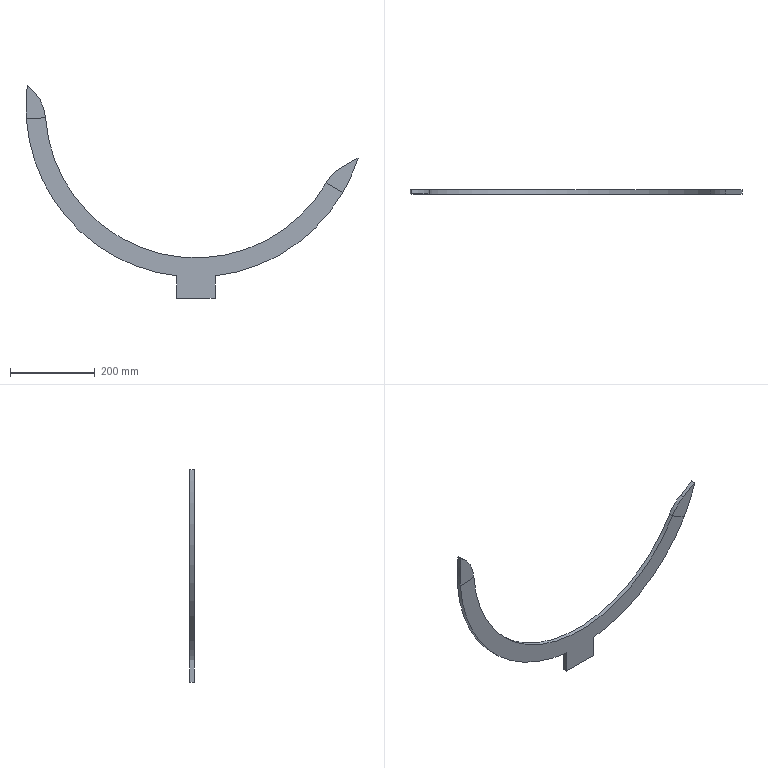Part | NX | features DATUM_CSYS 2, DIVIDE_FACE 1, EXTRUDE 1, SKETCH 1 | 1 solid | 15 faces | box 781.576 x 10 x 500 mm | volume 527562 mm3 | plane 10 | cylinder 5 | commonest cylinder face diameters 200 x2 800 x2 710 x1
STEP:
#1=CARTESIAN_POINT('',(-354.112,-5.,-25.096));
#2=VERTEX_POINT('',#1);
#3=CARTESIAN_POINT('',(306.914,-5.,-178.406));
#4=VERTEX_POINT('',#3);
#5=CARTESIAN_POINT('',(0.,-5.,0.));
#6=DIRECTION('',(0.,1.,0.));
#7=DIRECTION('',(1.,0.,0.));
#8=AXIS2_PLACEMENT_3D('',#5,#6,#7);
#9=CIRCLE('',#8,355.);
#10=EDGE_CURVE('',#2,#4,#9,.F.);
#11=ORIENTED_EDGE('',*,*,#10,.F.);
#12=CARTESIAN_POINT('',(-398.999,-5.,-28.277));
#13=VERTEX_POINT('',#12);
#14=CARTESIAN_POINT('',(-354.112,-5.,-25.096));
#15=DIRECTION('',(-0.9975,0.,-0.07069));
#16=VECTOR('',#15,1000.);
#17=LINE('',#14,#16);
#18=EDGE_CURVE('',#2,#13,#17,.T.);
#19=ORIENTED_EDGE('',*,*,#18,.T.);
#20=CARTESIAN_POINT('',(-45.,-5.,-397.461));
#21=VERTEX_POINT('',#20);
#22=CARTESIAN_POINT('',(0.,-5.,0.));
#23=DIRECTION('',(0.,-1.,0.));
#24=DIRECTION('',(1.,0.,0.));
#25=AXIS2_PLACEMENT_3D('',#22,#23,#24);
#26=CIRCLE('',#25,400.);
#27=EDGE_CURVE('',#21,#13,#26,.F.);
#28=ORIENTED_EDGE('',*,*,#27,.F.);
#29=CARTESIAN_POINT('',(-45.,-5.,-450.));
#30=VERTEX_POINT('',#29);
#31=CARTESIAN_POINT('',(-45.,-5.,-397.461));
#32=DIRECTION('',(0.,0.,-1.));
#33=VECTOR('',#32,1000.);
#34=LINE('',#31,#33);
#35=EDGE_CURVE('',#30,#21,#34,.F.);
#36=ORIENTED_EDGE('',*,*,#35,.F.);
#37=CARTESIAN_POINT('',(45.,-5.,-450.));
#38=VERTEX_POINT('',#37);
#39=CARTESIAN_POINT('',(-45.,-5.,-450.));
#40=DIRECTION('',(1.,0.,0.));
#41=VECTOR('',#40,1000.);
#42=LINE('',#39,#41);
#43=EDGE_CURVE('',#38,#30,#42,.F.);
#44=ORIENTED_EDGE('',*,*,#43,.F.);
#45=CARTESIAN_POINT('',(45.,-5.,-397.461));
#46=VERTEX_POINT('',#45);
#47=CARTESIAN_POINT('',(45.,-5.,-450.));
#48=DIRECTION('',(0.,0.,1.));
#49=VECTOR('',#48,1000.);
#50=LINE('',#47,#49);
#51=EDGE_CURVE('',#46,#38,#50,.F.);
#52=ORIENTED_EDGE('',*,*,#51,.F.);
#53=CARTESIAN_POINT('',(345.819,-5.,-201.021));
#54=VERTEX_POINT('',#53);
#55=CARTESIAN_POINT('',(0.,-5.,0.));
#56=DIRECTION('',(0.,-1.,0.));
#57=DIRECTION('',(1.,0.,0.));
#58=AXIS2_PLACEMENT_3D('',#55,#56,#57);
#59=CIRCLE('',#58,400.);
#60=EDGE_CURVE('',#54,#46,#59,.F.);
#61=ORIENTED_EDGE('',*,*,#60,.F.);
#62=CARTESIAN_POINT('',(345.819,-5.,-201.021));
#63=DIRECTION('',(-0.8645,0.,0.5026));
#64=VECTOR('',#63,1000.);
#65=LINE('',#62,#64);
#66=EDGE_CURVE('',#54,#4,#65,.T.);
#67=ORIENTED_EDGE('',*,*,#66,.T.);
#68=EDGE_LOOP('',(#11,#19,#28,#36,#44,#52,#61,#67));
#69=FACE_BOUND('',#68,.T.);
#70=CARTESIAN_POINT('',(-453.862,-5.,-32.165));
#71=DIRECTION('',(0.,-1.,0.));
#72=DIRECTION('',(0.,0.,-1.));
#73=AXIS2_PLACEMENT_3D('',#70,#71,#72);
#74=PLANE('',#73);
#75=ADVANCED_FACE('',(#69),#74,.T.);
#76=ORIENTED_EDGE('',*,*,#18,.F.);
#77=CARTESIAN_POINT('',(-396.863,-5.,50.));
#78=VERTEX_POINT('',#77);
#79=CARTESIAN_POINT('',(-453.862,-5.,-32.165));
#80=DIRECTION('',(0.,-1.,0.));
#81=DIRECTION('',(1.,0.,0.));
#82=AXIS2_PLACEMENT_3D('',#79,#80,#81);
#83=CIRCLE('',#82,100.);
#84=EDGE_CURVE('',#78,#2,#83,.F.);
#85=ORIENTED_EDGE('',*,*,#84,.F.);
#86=CARTESIAN_POINT('',(0.,-5.,0.));
#87=DIRECTION('',(0.,-1.,0.));
#88=DIRECTION('',(1.,0.,0.));
#89=AXIS2_PLACEMENT_3D('',#86,#87,#88);
#90=CIRCLE('',#89,400.);
#91=EDGE_CURVE('',#13,#78,#90,.F.);
#92=ORIENTED_EDGE('',*,*,#91,.F.);
#93=EDGE_LOOP('',(#76,#85,#92));
#94=FACE_BOUND('',#93,.T.);
#95=CARTESIAN_POINT('',(-453.862,-5.,-32.165));
#96=DIRECTION('',(0.,-1.,0.));
#97=DIRECTION('',(0.,0.,-1.));
#98=AXIS2_PLACEMENT_3D('',#95,#96,#97);
#99=PLANE('',#98);
#100=ADVANCED_FACE('',(#94),#99,.T.);
#101=CARTESIAN_POINT('',(-396.863,5.,50.));
#102=VERTEX_POINT('',#101);
#103=CARTESIAN_POINT('',(-354.112,5.,-25.096));
#104=VERTEX_POINT('',#103);
#105=CARTESIAN_POINT('',(-453.862,5.,-32.165));
#106=DIRECTION('',(0.,-1.,0.));
#107=DIRECTION('',(1.,0.,0.));
#108=AXIS2_PLACEMENT_3D('',#105,#106,#107);
#109=CIRCLE('',#108,100.);
#110=EDGE_CURVE('',#102,#104,#109,.F.);
#111=ORIENTED_EDGE('',*,*,#110,.T.);
#112=CARTESIAN_POINT('',(-398.999,5.,-28.277));
#113=VERTEX_POINT('',#112);
#114=CARTESIAN_POINT('',(-354.112,5.,-25.096));
#115=DIRECTION('',(-0.9975,0.,-0.07069));
#116=VECTOR('',#115,1000.);
#117=LINE('',#114,#116);
#118=EDGE_CURVE('',#104,#113,#117,.T.);
#119=ORIENTED_EDGE('',*,*,#118,.T.);
#120=CARTESIAN_POINT('',(0.,5.,0.));
#121=DIRECTION('',(0.,-1.,0.));
#122=DIRECTION('',(1.,0.,0.));
#123=AXIS2_PLACEMENT_3D('',#120,#121,#122);
#124=CIRCLE('',#123,400.);
#125=EDGE_CURVE('',#113,#102,#124,.F.);
#126=ORIENTED_EDGE('',*,*,#125,.T.);
#127=EDGE_LOOP('',(#111,#119,#126));
#128=FACE_BOUND('',#127,.T.);
#129=CARTESIAN_POINT('',(-453.862,5.,-32.165));
#130=DIRECTION('',(0.,-1.,0.));
#131=DIRECTION('',(0.,0.,-1.));
#132=AXIS2_PLACEMENT_3D('',#129,#130,#131);
#133=PLANE('',#132);
#134=ADVANCED_FACE('',(#128),#133,.F.);
#135=CARTESIAN_POINT('',(381.576,5.,-120.));
#136=VERTEX_POINT('',#135);
#137=CARTESIAN_POINT('',(345.819,5.,-201.021));
#138=VERTEX_POINT('',#137);
#139=CARTESIAN_POINT('',(0.,5.,0.));
#140=DIRECTION('',(0.,-1.,0.));
#141=DIRECTION('',(1.,0.,0.));
#142=AXIS2_PLACEMENT_3D('',#139,#140,#141);
#143=CIRCLE('',#142,400.);
#144=EDGE_CURVE('',#136,#138,#143,.F.);
#145=ORIENTED_EDGE('',*,*,#144,.T.);
#146=CARTESIAN_POINT('',(306.914,5.,-178.406));
#147=VERTEX_POINT('',#146);
#148=CARTESIAN_POINT('',(345.819,5.,-201.021));
#149=DIRECTION('',(-0.8645,0.,0.5026));
#150=VECTOR('',#149,1000.);
#151=LINE('',#148,#150);
#152=EDGE_CURVE('',#138,#147,#151,.T.);
#153=ORIENTED_EDGE('',*,*,#152,.T.);
#154=CARTESIAN_POINT('',(343.369,5.,-142.059));
#155=VERTEX_POINT('',#154);
#156=CARTESIAN_POINT('',(393.369,5.,-228.661));
#157=DIRECTION('',(0.,-1.,0.));
#158=DIRECTION('',(1.,0.,0.));
#159=AXIS2_PLACEMENT_3D('',#156,#157,#158);
#160=CIRCLE('',#159,100.);
#161=EDGE_CURVE('',#147,#155,#160,.F.);
#162=ORIENTED_EDGE('',*,*,#161,.T.);
#163=CARTESIAN_POINT('',(381.576,5.,-120.));
#164=DIRECTION('',(-0.866,0.,-0.5));
#165=VECTOR('',#164,1000.);
#166=LINE('',#163,#165);
#167=EDGE_CURVE('',#155,#136,#166,.F.);
#168=ORIENTED_EDGE('',*,*,#167,.T.);
#169=EDGE_LOOP('',(#145,#153,#162,#168));
#170=FACE_BOUND('',#169,.T.);
#171=CARTESIAN_POINT('',(-453.862,5.,-32.165));
#172=DIRECTION('',(0.,-1.,0.));
#173=DIRECTION('',(0.,0.,-1.));
#174=AXIS2_PLACEMENT_3D('',#171,#172,#173);
#175=PLANE('',#174);
#176=ADVANCED_FACE('',(#170),#175,.F.);
#177=ORIENTED_EDGE('',*,*,#110,.F.);
#178=CARTESIAN_POINT('',(-396.863,-5.,50.));
#179=DIRECTION('',(0.,1.,0.));
#180=VECTOR('',#179,1000.);
#181=LINE('',#178,#180);
#182=EDGE_CURVE('',#78,#102,#181,.T.);
#183=ORIENTED_EDGE('',*,*,#182,.F.);
#184=ORIENTED_EDGE('',*,*,#84,.T.);
#185=CARTESIAN_POINT('',(-354.112,-5.,-25.096));
#186=DIRECTION('',(0.,1.,0.));
#187=VECTOR('',#186,1000.);
#188=LINE('',#185,#187);
#189=EDGE_CURVE('',#2,#104,#188,.T.);
#190=ORIENTED_EDGE('',*,*,#189,.T.);
#191=EDGE_LOOP('',(#177,#183,#184,#190));
#192=FACE_BOUND('',#191,.T.);
#193=CARTESIAN_POINT('',(-453.862,-5.,-32.165));
#194=DIRECTION('',(0.,1.,0.));
#195=DIRECTION('',(0.,0.,1.));
#196=AXIS2_PLACEMENT_3D('',#193,#194,#195);
#197=CYLINDRICAL_SURFACE('',#196,100.);
#198=ADVANCED_FACE('',(#192),#197,.T.);
#199=CARTESIAN_POINT('',(-45.,5.,-397.461));
#200=VERTEX_POINT('',#199);
#201=CARTESIAN_POINT('',(0.,5.,0.));
#202=DIRECTION('',(0.,-1.,0.));
#203=DIRECTION('',(1.,0.,0.));
#204=AXIS2_PLACEMENT_3D('',#201,#202,#203);
#205=CIRCLE('',#204,400.);
#206=EDGE_CURVE('',#200,#113,#205,.F.);
#207=ORIENTED_EDGE('',*,*,#206,.F.);
#208=CARTESIAN_POINT('',(-45.,-5.,-397.461));
#209=DIRECTION('',(0.,1.,0.));
#210=VECTOR('',#209,1000.);
#211=LINE('',#208,#210);
#212=EDGE_CURVE('',#21,#200,#211,.T.);
#213=ORIENTED_EDGE('',*,*,#212,.F.);
#214=ORIENTED_EDGE('',*,*,#27,.T.);
#215=ORIENTED_EDGE('',*,*,#91,.T.);
#216=ORIENTED_EDGE('',*,*,#182,.T.);
#217=ORIENTED_EDGE('',*,*,#125,.F.);
#218=EDGE_LOOP('',(#207,#213,#214,#215,#216,#217));
#219=FACE_BOUND('',#218,.T.);
#220=CARTESIAN_POINT('',(0.,-5.,0.));
#221=DIRECTION('',(0.,1.,0.));
#222=DIRECTION('',(0.,0.,1.));
#223=AXIS2_PLACEMENT_3D('',#220,#221,#222);
#224=CYLINDRICAL_SURFACE('',#223,400.);
#225=ADVANCED_FACE('',(#219),#224,.T.);
#226=CARTESIAN_POINT('',(-45.,5.,-450.));
#227=VERTEX_POINT('',#226);
#228=CARTESIAN_POINT('',(-45.,5.,-397.461));
#229=DIRECTION('',(0.,0.,-1.));
#230=VECTOR('',#229,1000.);
#231=LINE('',#228,#230);
#232=EDGE_CURVE('',#227,#200,#231,.F.);
#233=ORIENTED_EDGE('',*,*,#232,.F.);
#234=CARTESIAN_POINT('',(-45.,-5.,-450.));
#235=DIRECTION('',(0.,1.,0.));
#236=VECTOR('',#235,1000.);
#237=LINE('',#234,#236);
#238=EDGE_CURVE('',#30,#227,#237,.T.);
#239=ORIENTED_EDGE('',*,*,#238,.F.);
#240=ORIENTED_EDGE('',*,*,#35,.T.);
#241=ORIENTED_EDGE('',*,*,#212,.T.);
#242=EDGE_LOOP('',(#233,#239,#240,#241));
#243=FACE_BOUND('',#242,.T.);
#244=CARTESIAN_POINT('',(-45.,-5.,-397.461));
#245=DIRECTION('',(1.,0.,0.));
#246=DIRECTION('',(0.,0.,-1.));
#247=AXIS2_PLACEMENT_3D('',#244,#245,#246);
#248=PLANE('',#247);
#249=ADVANCED_FACE('',(#243),#248,.F.);
#250=CARTESIAN_POINT('',(45.,5.,-450.));
#251=VERTEX_POINT('',#250);
#252=CARTESIAN_POINT('',(-45.,5.,-450.));
#253=DIRECTION('',(1.,0.,0.));
#254=VECTOR('',#253,1000.);
#255=LINE('',#252,#254);
#256=EDGE_CURVE('',#251,#227,#255,.F.);
#257=ORIENTED_EDGE('',*,*,#256,.F.);
#258=CARTESIAN_POINT('',(45.,-5.,-450.));
#259=DIRECTION('',(0.,1.,0.));
#260=VECTOR('',#259,1000.);
#261=LINE('',#258,#260);
#262=EDGE_CURVE('',#38,#251,#261,.T.);
#263=ORIENTED_EDGE('',*,*,#262,.F.);
#264=ORIENTED_EDGE('',*,*,#43,.T.);
#265=ORIENTED_EDGE('',*,*,#238,.T.);
#266=EDGE_LOOP('',(#257,#263,#264,#265));
#267=FACE_BOUND('',#266,.T.);
#268=CARTESIAN_POINT('',(-45.,-5.,-450.));
#269=DIRECTION('',(0.,0.,1.));
#270=DIRECTION('',(1.,0.,0.));
#271=AXIS2_PLACEMENT_3D('',#268,#269,#270);
#272=PLANE('',#271);
#273=ADVANCED_FACE('',(#267),#272,.F.);
#274=CARTESIAN_POINT('',(45.,5.,-397.461));
#275=VERTEX_POINT('',#274);
#276=CARTESIAN_POINT('',(45.,5.,-450.));
#277=DIRECTION('',(0.,0.,1.));
#278=VECTOR('',#277,1000.);
#279=LINE('',#276,#278);
#280=EDGE_CURVE('',#275,#251,#279,.F.);
#281=ORIENTED_EDGE('',*,*,#280,.F.);
#282=CARTESIAN_POINT('',(45.,-5.,-397.461));
#283=DIRECTION('',(0.,1.,0.));
#284=VECTOR('',#283,1000.);
#285=LINE('',#282,#284);
#286=EDGE_CURVE('',#46,#275,#285,.T.);
#287=ORIENTED_EDGE('',*,*,#286,.F.);
#288=ORIENTED_EDGE('',*,*,#51,.T.);
#289=ORIENTED_EDGE('',*,*,#262,.T.);
#290=EDGE_LOOP('',(#281,#287,#288,#289));
#291=FACE_BOUND('',#290,.T.);
#292=CARTESIAN_POINT('',(45.,-5.,-450.));
#293=DIRECTION('',(-1.,0.,0.));
#294=DIRECTION('',(0.,0.,1.));
#295=AXIS2_PLACEMENT_3D('',#292,#293,#294);
#296=PLANE('',#295);
#297=ADVANCED_FACE('',(#291),#296,.F.);
#298=ORIENTED_EDGE('',*,*,#144,.F.);
#299=CARTESIAN_POINT('',(381.576,-5.,-120.));
#300=VERTEX_POINT('',#299);
#301=CARTESIAN_POINT('',(381.576,-5.,-120.));
#302=DIRECTION('',(0.,1.,0.));
#303=VECTOR('',#302,1000.);
#304=LINE('',#301,#303);
#305=EDGE_CURVE('',#300,#136,#304,.T.);
#306=ORIENTED_EDGE('',*,*,#305,.F.);
#307=CARTESIAN_POINT('',(0.,-5.,0.));
#308=DIRECTION('',(0.,-1.,0.));
#309=DIRECTION('',(1.,0.,0.));
#310=AXIS2_PLACEMENT_3D('',#307,#308,#309);
#311=CIRCLE('',#310,400.);
#312=EDGE_CURVE('',#300,#54,#311,.F.);
#313=ORIENTED_EDGE('',*,*,#312,.T.);
#314=ORIENTED_EDGE('',*,*,#60,.T.);
#315=ORIENTED_EDGE('',*,*,#286,.T.);
#316=CARTESIAN_POINT('',(0.,5.,0.));
#317=DIRECTION('',(0.,-1.,0.));
#318=DIRECTION('',(1.,0.,0.));
#319=AXIS2_PLACEMENT_3D('',#316,#317,#318);
#320=CIRCLE('',#319,400.);
#321=EDGE_CURVE('',#138,#275,#320,.F.);
#322=ORIENTED_EDGE('',*,*,#321,.F.);
#323=EDGE_LOOP('',(#298,#306,#313,#314,#315,#322));
#324=FACE_BOUND('',#323,.T.);
#325=CARTESIAN_POINT('',(0.,-5.,0.));
#326=DIRECTION('',(0.,1.,0.));
#327=DIRECTION('',(0.,0.,1.));
#328=AXIS2_PLACEMENT_3D('',#325,#326,#327);
#329=CYLINDRICAL_SURFACE('',#328,400.);
#330=ADVANCED_FACE('',(#324),#329,.T.);
#331=ORIENTED_EDGE('',*,*,#167,.F.);
#332=CARTESIAN_POINT('',(343.369,-5.,-142.059));
#333=VERTEX_POINT('',#332);
#334=CARTESIAN_POINT('',(343.369,-5.,-142.059));
#335=DIRECTION('',(0.,1.,0.));
#336=VECTOR('',#335,1000.);
#337=LINE('',#334,#336);
#338=EDGE_CURVE('',#333,#155,#337,.T.);
#339=ORIENTED_EDGE('',*,*,#338,.F.);
#340=CARTESIAN_POINT('',(381.576,-5.,-120.));
#341=DIRECTION('',(-0.866,0.,-0.5));
#342=VECTOR('',#341,1000.);
#343=LINE('',#340,#342);
#344=EDGE_CURVE('',#333,#300,#343,.F.);
#345=ORIENTED_EDGE('',*,*,#344,.T.);
#346=ORIENTED_EDGE('',*,*,#305,.T.);
#347=EDGE_LOOP('',(#331,#339,#345,#346));
#348=FACE_BOUND('',#347,.T.);
#349=CARTESIAN_POINT('',(381.576,-5.,-120.));
#350=DIRECTION('',(0.5,0.,-0.866));
#351=DIRECTION('',(-0.866,0.,-0.5));
#352=AXIS2_PLACEMENT_3D('',#349,#350,#351);
#353=PLANE('',#352);
#354=ADVANCED_FACE('',(#348),#353,.F.);
#355=ORIENTED_EDGE('',*,*,#161,.F.);
#356=CARTESIAN_POINT('',(306.914,-5.,-178.406));
#357=DIRECTION('',(0.,1.,0.));
#358=VECTOR('',#357,1000.);
#359=LINE('',#356,#358);
#360=EDGE_CURVE('',#4,#147,#359,.T.);
#361=ORIENTED_EDGE('',*,*,#360,.F.);
#362=CARTESIAN_POINT('',(393.369,-5.,-228.661));
#363=DIRECTION('',(0.,-1.,0.));
#364=DIRECTION('',(1.,0.,0.));
#365=AXIS2_PLACEMENT_3D('',#362,#363,#364);
#366=CIRCLE('',#365,100.);
#367=EDGE_CURVE('',#4,#333,#366,.F.);
#368=ORIENTED_EDGE('',*,*,#367,.T.);
#369=ORIENTED_EDGE('',*,*,#338,.T.);
#370=EDGE_LOOP('',(#355,#361,#368,#369));
#371=FACE_BOUND('',#370,.T.);
#372=CARTESIAN_POINT('',(393.369,-5.,-228.661));
#373=DIRECTION('',(0.,1.,0.));
#374=DIRECTION('',(0.,0.,1.));
#375=AXIS2_PLACEMENT_3D('',#372,#373,#374);
#376=CYLINDRICAL_SURFACE('',#375,100.);
#377=ADVANCED_FACE('',(#371),#376,.T.);
#378=CARTESIAN_POINT('',(0.,5.,0.));
#379=DIRECTION('',(0.,1.,0.));
#380=DIRECTION('',(1.,0.,0.));
#381=AXIS2_PLACEMENT_3D('',#378,#379,#380);
#382=CIRCLE('',#381,355.);
#383=EDGE_CURVE('',#104,#147,#382,.F.);
#384=ORIENTED_EDGE('',*,*,#383,.F.);
#385=ORIENTED_EDGE('',*,*,#189,.F.);
#386=ORIENTED_EDGE('',*,*,#10,.T.);
#387=ORIENTED_EDGE('',*,*,#360,.T.);
#388=EDGE_LOOP('',(#384,#385,#386,#387));
#389=FACE_BOUND('',#388,.T.);
#390=CARTESIAN_POINT('',(0.,-5.,0.));
#391=DIRECTION('',(0.,1.,0.));
#392=DIRECTION('',(0.,0.,1.));
#393=AXIS2_PLACEMENT_3D('',#390,#391,#392);
#394=CYLINDRICAL_SURFACE('',#393,355.);
#395=ADVANCED_FACE('',(#389),#394,.F.);
#396=ORIENTED_EDGE('',*,*,#66,.F.);
#397=ORIENTED_EDGE('',*,*,#312,.F.);
#398=ORIENTED_EDGE('',*,*,#344,.F.);
#399=ORIENTED_EDGE('',*,*,#367,.F.);
#400=EDGE_LOOP('',(#396,#397,#398,#399));
#401=FACE_BOUND('',#400,.T.);
#402=CARTESIAN_POINT('',(-453.862,-5.,-32.165));
#403=DIRECTION('',(0.,-1.,0.));
#404=DIRECTION('',(0.,0.,-1.));
#405=AXIS2_PLACEMENT_3D('',#402,#403,#404);
#406=PLANE('',#405);
#407=ADVANCED_FACE('',(#401),#406,.T.);
#408=ORIENTED_EDGE('',*,*,#118,.F.);
#409=ORIENTED_EDGE('',*,*,#383,.T.);
#410=ORIENTED_EDGE('',*,*,#152,.F.);
#411=ORIENTED_EDGE('',*,*,#321,.T.);
#412=ORIENTED_EDGE('',*,*,#280,.T.);
#413=ORIENTED_EDGE('',*,*,#256,.T.);
#414=ORIENTED_EDGE('',*,*,#232,.T.);
#415=ORIENTED_EDGE('',*,*,#206,.T.);
#416=EDGE_LOOP('',(#408,#409,#410,#411,#412,#413,#414,#415));
#417=FACE_BOUND('',#416,.T.);
#418=CARTESIAN_POINT('',(-453.862,5.,-32.165));
#419=DIRECTION('',(0.,-1.,0.));
#420=DIRECTION('',(0.,0.,-1.));
#421=AXIS2_PLACEMENT_3D('',#418,#419,#420);
#422=PLANE('',#421);
#423=ADVANCED_FACE('',(#417),#422,.F.);
#424=CLOSED_SHELL('',(#75,#100,#134,#176,#198,#225,#249,#273,#297,#330,#354,#377,#395,#407,#423));
#425=MANIFOLD_SOLID_BREP('',#424);
#426=(LENGTH_UNIT()NAMED_UNIT(*)SI_UNIT(.MILLI.,.METRE.));
#427=UNCERTAINTY_MEASURE_WITH_UNIT(LENGTH_MEASURE(0.00001),#426,'','');
#428=(NAMED_UNIT(*)PLANE_ANGLE_UNIT()SI_UNIT($,.RADIAN.));
#429=(NAMED_UNIT(*)SI_UNIT($,.STERADIAN.)SOLID_ANGLE_UNIT());
#430=(GEOMETRIC_REPRESENTATION_CONTEXT(3)GLOBAL_UNCERTAINTY_ASSIGNED_CONTEXT((#427))GLOBAL_UNIT_ASSIGNED_CONTEXT((#426,#428,#429))REPRESENTATION_CONTEXT('',''));
#431=ADVANCED_BREP_SHAPE_REPRESENTATION('',(#425),#430);